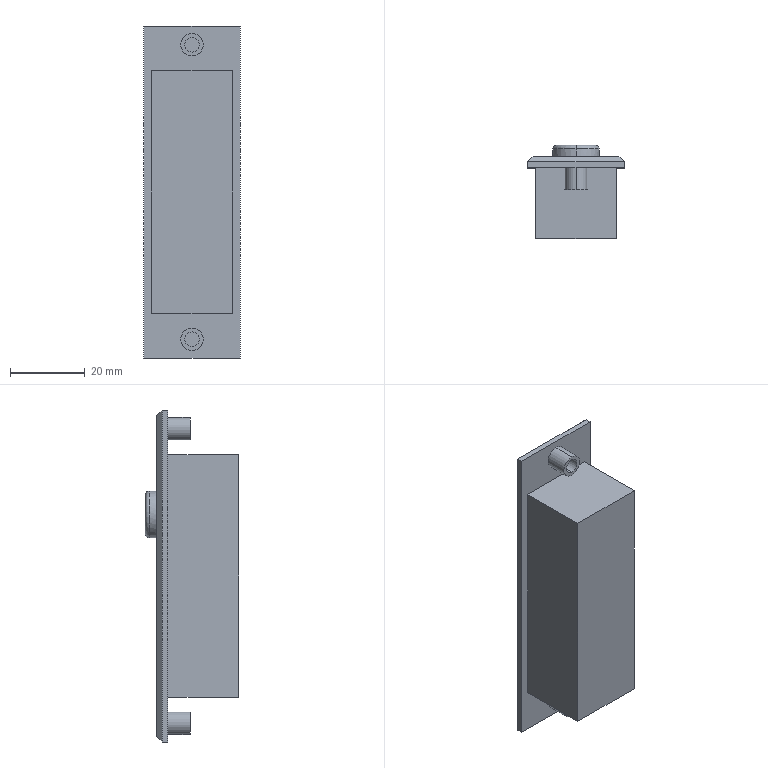Part | SolidWorks | features ICE 2, BossThin 1, Chamfer 1, CutThin 1, Extrusion 1, Fillet 1 | 1 solid | 45 faces | box 26 x 25 x 89 mm | volume 33780 mm3 | plane 29 | cylinder 10 | cone 4 | torus 2 | commonest cylinder face diameters 4 x4 6 x4 12.5 x2
STEP:
#1=CARTESIAN_POINT('',(0.,-6.,41.5));
#2=VERTEX_POINT('',#1);
#3=CARTESIAN_POINT('',(0.,-6.,37.5));
#4=VERTEX_POINT('',#3);
#5=CARTESIAN_POINT('',(0.,-6.,39.5));
#6=DIRECTION('',(0.,-1.,0.));
#7=DIRECTION('',(1.,0.,0.));
#8=AXIS2_PLACEMENT_3D('',#5,#6,#7);
#9=CIRCLE('',#8,2.);
#10=EDGE_CURVE('',#2,#4,#9,.T.);
#11=ORIENTED_EDGE('',*,*,#10,.T.);
#12=CARTESIAN_POINT('',(0.,0.,37.5));
#13=VERTEX_POINT('',#12);
#14=CARTESIAN_POINT('',(0.,-6.,37.5));
#15=DIRECTION('',(0.,1.,0.));
#16=VECTOR('',#15,1000.);
#17=LINE('',#14,#16);
#18=EDGE_CURVE('',#4,#13,#17,.T.);
#19=ORIENTED_EDGE('',*,*,#18,.T.);
#20=CARTESIAN_POINT('',(0.,0.,41.5));
#21=VERTEX_POINT('',#20);
#22=CARTESIAN_POINT('',(0.,0.,39.5));
#23=DIRECTION('',(0.,-1.,0.));
#24=DIRECTION('',(1.,0.,0.));
#25=AXIS2_PLACEMENT_3D('',#22,#23,#24);
#26=CIRCLE('',#25,2.);
#27=EDGE_CURVE('',#21,#13,#26,.T.);
#28=ORIENTED_EDGE('',*,*,#27,.F.);
#29=CARTESIAN_POINT('',(0.,-6.,41.5));
#30=DIRECTION('',(0.,1.,0.));
#31=VECTOR('',#30,1000.);
#32=LINE('',#29,#31);
#33=EDGE_CURVE('',#2,#21,#32,.T.);
#34=ORIENTED_EDGE('',*,*,#33,.F.);
#35=EDGE_LOOP('',(#11,#19,#28,#34));
#36=FACE_OUTER_BOUND('',#35,.T.);
#37=CARTESIAN_POINT('',(0.,-6.,39.5));
#38=DIRECTION('',(0.,1.,0.));
#39=DIRECTION('',(0.,0.,1.));
#40=AXIS2_PLACEMENT_3D('',#37,#38,#39);
#41=CYLINDRICAL_SURFACE('',#40,2.);
#42=ADVANCED_FACE('',(#36),#41,.F.);
#43=CARTESIAN_POINT('',(0.,-6.,36.5));
#44=VERTEX_POINT('',#43);
#45=CARTESIAN_POINT('',(0.,-6.,42.5));
#46=VERTEX_POINT('',#45);
#47=CARTESIAN_POINT('',(0.,-6.,39.5));
#48=DIRECTION('',(0.,-1.,0.));
#49=DIRECTION('',(0.,0.,-1.));
#50=AXIS2_PLACEMENT_3D('',#47,#48,#49);
#51=CIRCLE('',#50,3.);
#52=EDGE_CURVE('',#44,#46,#51,.T.);
#53=ORIENTED_EDGE('',*,*,#52,.F.);
#54=CARTESIAN_POINT('',(0.,0.,36.5));
#55=VERTEX_POINT('',#54);
#56=CARTESIAN_POINT('',(0.,-6.,36.5));
#57=DIRECTION('',(0.,1.,0.));
#58=VECTOR('',#57,1000.);
#59=LINE('',#56,#58);
#60=EDGE_CURVE('',#44,#55,#59,.T.);
#61=ORIENTED_EDGE('',*,*,#60,.T.);
#62=CARTESIAN_POINT('',(0.,0.,42.5));
#63=VERTEX_POINT('',#62);
#64=CARTESIAN_POINT('',(0.,0.,39.5));
#65=DIRECTION('',(0.,-1.,0.));
#66=DIRECTION('',(0.,0.,1.));
#67=AXIS2_PLACEMENT_3D('',#64,#65,#66);
#68=CIRCLE('',#67,3.);
#69=EDGE_CURVE('',#55,#63,#68,.T.);
#70=ORIENTED_EDGE('',*,*,#69,.T.);
#71=CARTESIAN_POINT('',(0.,-6.,42.5));
#72=DIRECTION('',(0.,1.,0.));
#73=VECTOR('',#72,1000.);
#74=LINE('',#71,#73);
#75=EDGE_CURVE('',#46,#63,#74,.T.);
#76=ORIENTED_EDGE('',*,*,#75,.F.);
#77=EDGE_LOOP('',(#53,#61,#70,#76));
#78=FACE_OUTER_BOUND('',#77,.T.);
#79=CARTESIAN_POINT('',(0.,-6.,39.5));
#80=DIRECTION('',(0.,1.,0.));
#81=DIRECTION('',(0.,0.,1.));
#82=AXIS2_PLACEMENT_3D('',#79,#80,#81);
#83=CYLINDRICAL_SURFACE('',#82,3.);
#84=ADVANCED_FACE('',(#78),#83,.T.);
#85=CARTESIAN_POINT('',(0.,-6.,-37.5));
#86=VERTEX_POINT('',#85);
#87=CARTESIAN_POINT('',(0.,-6.,-41.5));
#88=VERTEX_POINT('',#87);
#89=CARTESIAN_POINT('',(0.,-6.,-39.5));
#90=DIRECTION('',(0.,-1.,0.));
#91=DIRECTION('',(1.,0.,0.));
#92=AXIS2_PLACEMENT_3D('',#89,#90,#91);
#93=CIRCLE('',#92,2.);
#94=EDGE_CURVE('',#86,#88,#93,.T.);
#95=ORIENTED_EDGE('',*,*,#94,.T.);
#96=CARTESIAN_POINT('',(0.,0.,-41.5));
#97=VERTEX_POINT('',#96);
#98=CARTESIAN_POINT('',(0.,-6.,-41.5));
#99=DIRECTION('',(0.,1.,0.));
#100=VECTOR('',#99,1000.);
#101=LINE('',#98,#100);
#102=EDGE_CURVE('',#88,#97,#101,.T.);
#103=ORIENTED_EDGE('',*,*,#102,.T.);
#104=CARTESIAN_POINT('',(0.,0.,-37.5));
#105=VERTEX_POINT('',#104);
#106=CARTESIAN_POINT('',(0.,0.,-39.5));
#107=DIRECTION('',(0.,-1.,0.));
#108=DIRECTION('',(1.,0.,0.));
#109=AXIS2_PLACEMENT_3D('',#106,#107,#108);
#110=CIRCLE('',#109,2.);
#111=EDGE_CURVE('',#105,#97,#110,.T.);
#112=ORIENTED_EDGE('',*,*,#111,.F.);
#113=CARTESIAN_POINT('',(0.,-6.,-37.5));
#114=DIRECTION('',(0.,1.,0.));
#115=VECTOR('',#114,1000.);
#116=LINE('',#113,#115);
#117=EDGE_CURVE('',#86,#105,#116,.T.);
#118=ORIENTED_EDGE('',*,*,#117,.F.);
#119=EDGE_LOOP('',(#95,#103,#112,#118));
#120=FACE_OUTER_BOUND('',#119,.T.);
#121=CARTESIAN_POINT('',(0.,-6.,-39.5));
#122=DIRECTION('',(0.,1.,0.));
#123=DIRECTION('',(0.,0.,1.));
#124=AXIS2_PLACEMENT_3D('',#121,#122,#123);
#125=CYLINDRICAL_SURFACE('',#124,2.);
#126=ADVANCED_FACE('',(#120),#125,.F.);
#127=CARTESIAN_POINT('',(0.,-6.,-42.5));
#128=VERTEX_POINT('',#127);
#129=CARTESIAN_POINT('',(0.,-6.,-36.5));
#130=VERTEX_POINT('',#129);
#131=CARTESIAN_POINT('',(0.,-6.,-39.5));
#132=DIRECTION('',(0.,-1.,0.));
#133=DIRECTION('',(0.,0.,-1.));
#134=AXIS2_PLACEMENT_3D('',#131,#132,#133);
#135=CIRCLE('',#134,3.);
#136=EDGE_CURVE('',#128,#130,#135,.T.);
#137=ORIENTED_EDGE('',*,*,#136,.F.);
#138=CARTESIAN_POINT('',(0.,0.,-42.5));
#139=VERTEX_POINT('',#138);
#140=CARTESIAN_POINT('',(0.,-6.,-42.5));
#141=DIRECTION('',(0.,1.,0.));
#142=VECTOR('',#141,1000.);
#143=LINE('',#140,#142);
#144=EDGE_CURVE('',#128,#139,#143,.T.);
#145=ORIENTED_EDGE('',*,*,#144,.T.);
#146=CARTESIAN_POINT('',(0.,0.,-36.5));
#147=VERTEX_POINT('',#146);
#148=CARTESIAN_POINT('',(0.,0.,-39.5));
#149=DIRECTION('',(0.,-1.,0.));
#150=DIRECTION('',(0.,0.,1.));
#151=AXIS2_PLACEMENT_3D('',#148,#149,#150);
#152=CIRCLE('',#151,3.);
#153=EDGE_CURVE('',#139,#147,#152,.T.);
#154=ORIENTED_EDGE('',*,*,#153,.T.);
#155=CARTESIAN_POINT('',(0.,-6.,-36.5));
#156=DIRECTION('',(0.,1.,0.));
#157=VECTOR('',#156,1000.);
#158=LINE('',#155,#157);
#159=EDGE_CURVE('',#130,#147,#158,.T.);
#160=ORIENTED_EDGE('',*,*,#159,.F.);
#161=EDGE_LOOP('',(#137,#145,#154,#160));
#162=FACE_OUTER_BOUND('',#161,.T.);
#163=CARTESIAN_POINT('',(0.,-6.,-39.5));
#164=DIRECTION('',(0.,1.,0.));
#165=DIRECTION('',(0.,0.,1.));
#166=AXIS2_PLACEMENT_3D('',#163,#164,#165);
#167=CYLINDRICAL_SURFACE('',#166,3.);
#168=ADVANCED_FACE('',(#162),#167,.T.);
#169=CARTESIAN_POINT('',(0.,5.,10.25));
#170=VERTEX_POINT('',#169);
#171=CARTESIAN_POINT('',(0.,5.,22.75));
#172=VERTEX_POINT('',#171);
#173=CARTESIAN_POINT('',(0.,5.,16.5));
#174=DIRECTION('',(0.,-1.,0.));
#175=DIRECTION('',(0.,0.,1.));
#176=AXIS2_PLACEMENT_3D('',#173,#174,#175);
#177=CIRCLE('',#176,6.25);
#178=EDGE_CURVE('',#170,#172,#177,.T.);
#179=ORIENTED_EDGE('',*,*,#178,.F.);
#180=CARTESIAN_POINT('',(0.,6.,11.25));
#181=VERTEX_POINT('',#180);
#182=CARTESIAN_POINT('',(0.,5.,11.25));
#183=DIRECTION('',(1.,0.,0.));
#184=DIRECTION('',(0.,0.,-1.));
#185=AXIS2_PLACEMENT_3D('',#182,#183,#184);
#186=CIRCLE('',#185,1.);
#187=EDGE_CURVE('',#170,#181,#186,.T.);
#188=ORIENTED_EDGE('',*,*,#187,.T.);
#189=CARTESIAN_POINT('',(0.,6.,21.75));
#190=VERTEX_POINT('',#189);
#191=CARTESIAN_POINT('',(0.,6.,16.5));
#192=DIRECTION('',(0.,1.,0.));
#193=DIRECTION('',(0.,0.,1.));
#194=AXIS2_PLACEMENT_3D('',#191,#192,#193);
#195=CIRCLE('',#194,5.25);
#196=EDGE_CURVE('',#190,#181,#195,.T.);
#197=ORIENTED_EDGE('',*,*,#196,.F.);
#198=CARTESIAN_POINT('',(0.,5.,21.75));
#199=DIRECTION('',(-1.,0.,0.));
#200=DIRECTION('',(0.,0.,1.));
#201=AXIS2_PLACEMENT_3D('',#198,#199,#200);
#202=CIRCLE('',#201,1.);
#203=EDGE_CURVE('',#172,#190,#202,.T.);
#204=ORIENTED_EDGE('',*,*,#203,.F.);
#205=EDGE_LOOP('',(#179,#188,#197,#204));
#206=FACE_OUTER_BOUND('',#205,.T.);
#207=CARTESIAN_POINT('',(0.,5.,16.5));
#208=DIRECTION('',(0.,1.,0.));
#209=DIRECTION('',(0.,0.,1.));
#210=AXIS2_PLACEMENT_3D('',#207,#208,#209);
#211=TOROIDAL_SURFACE('',#210,5.25,1.);
#212=ADVANCED_FACE('',(#206),#211,.T.);
#213=ORIENTED_EDGE('',*,*,#178,.T.);
#214=CARTESIAN_POINT('',(0.,3.,22.75));
#215=VERTEX_POINT('',#214);
#216=CARTESIAN_POINT('',(0.,6.,22.75));
#217=DIRECTION('',(0.,-1.,0.));
#218=VECTOR('',#217,1000.);
#219=LINE('',#216,#218);
#220=EDGE_CURVE('',#172,#215,#219,.T.);
#221=ORIENTED_EDGE('',*,*,#220,.T.);
#222=CARTESIAN_POINT('',(6.25,3.,16.5));
#223=VERTEX_POINT('',#222);
#224=CARTESIAN_POINT('',(0.,3.,16.5));
#225=DIRECTION('',(0.,1.,0.));
#226=DIRECTION('',(1.,0.,0.));
#227=AXIS2_PLACEMENT_3D('',#224,#225,#226);
#228=CIRCLE('',#227,6.25);
#229=EDGE_CURVE('',#215,#223,#228,.T.);
#230=ORIENTED_EDGE('',*,*,#229,.T.);
#231=CARTESIAN_POINT('',(0.,3.,10.25));
#232=VERTEX_POINT('',#231);
#233=CARTESIAN_POINT('',(0.,3.,16.5));
#234=DIRECTION('',(0.,1.,0.));
#235=DIRECTION('',(1.,0.,0.));
#236=AXIS2_PLACEMENT_3D('',#233,#234,#235);
#237=CIRCLE('',#236,6.25);
#238=EDGE_CURVE('',#223,#232,#237,.T.);
#239=ORIENTED_EDGE('',*,*,#238,.T.);
#240=CARTESIAN_POINT('',(0.,6.,10.25));
#241=DIRECTION('',(0.,-1.,0.));
#242=VECTOR('',#241,1000.);
#243=LINE('',#240,#242);
#244=EDGE_CURVE('',#170,#232,#243,.T.);
#245=ORIENTED_EDGE('',*,*,#244,.F.);
#246=EDGE_LOOP('',(#213,#221,#230,#239,#245));
#247=FACE_OUTER_BOUND('',#246,.T.);
#248=CARTESIAN_POINT('',(0.,6.,16.5));
#249=DIRECTION('',(0.,-1.,0.));
#250=DIRECTION('',(0.,0.,-1.));
#251=AXIS2_PLACEMENT_3D('',#248,#249,#250);
#252=CYLINDRICAL_SURFACE('',#251,6.25);
#253=ADVANCED_FACE('',(#247),#252,.T.);
#254=CARTESIAN_POINT('',(-6.25,3.,16.5));
#255=VERTEX_POINT('',#254);
#256=CARTESIAN_POINT('',(0.,3.,16.5));
#257=DIRECTION('',(0.,1.,0.));
#258=DIRECTION('',(1.,0.,0.));
#259=AXIS2_PLACEMENT_3D('',#256,#257,#258);
#260=CIRCLE('',#259,6.25);
#261=EDGE_CURVE('',#255,#215,#260,.T.);
#262=ORIENTED_EDGE('',*,*,#261,.F.);
#263=CARTESIAN_POINT('',(-6.5,2.741,16.5));
#264=VERTEX_POINT('',#263);
#265=CARTESIAN_POINT('',(-6.25,3.,16.5));
#266=DIRECTION('',(-0.6947,-0.7193,0.));
#267=VECTOR('',#266,1000.);
#268=LINE('',#265,#267);
#269=EDGE_CURVE('',#255,#264,#268,.T.);
#270=ORIENTED_EDGE('',*,*,#269,.T.);
#271=CARTESIAN_POINT('',(6.5,2.741,16.5));
#272=VERTEX_POINT('',#271);
#273=CARTESIAN_POINT('',(0.,2.741,16.5));
#274=DIRECTION('',(0.,1.,0.));
#275=DIRECTION('',(0.,0.,1.));
#276=AXIS2_PLACEMENT_3D('',#273,#274,#275);
#277=CIRCLE('',#276,6.5);
#278=EDGE_CURVE('',#264,#272,#277,.T.);
#279=ORIENTED_EDGE('',*,*,#278,.T.);
#280=CARTESIAN_POINT('',(6.25,3.,16.5));
#281=DIRECTION('',(0.6947,-0.7193,0.));
#282=VECTOR('',#281,1000.);
#283=LINE('',#280,#282);
#284=EDGE_CURVE('',#223,#272,#283,.T.);
#285=ORIENTED_EDGE('',*,*,#284,.F.);
#286=ORIENTED_EDGE('',*,*,#229,.F.);
#287=EDGE_LOOP('',(#262,#270,#279,#285,#286));
#288=FACE_OUTER_BOUND('',#287,.T.);
#289=CARTESIAN_POINT('',(0.,3.,16.5));
#290=DIRECTION('',(0.,-1.,0.));
#291=DIRECTION('',(1.,0.,0.));
#292=AXIS2_PLACEMENT_3D('',#289,#290,#291);
#293=CONICAL_SURFACE('',#292,6.25,0.7679);
#294=ADVANCED_FACE('',(#288),#293,.T.);
#295=ORIENTED_EDGE('',*,*,#278,.F.);
#296=CARTESIAN_POINT('',(-6.75,3.,16.5));
#297=VERTEX_POINT('',#296);
#298=CARTESIAN_POINT('',(-6.75,3.,16.5));
#299=DIRECTION('',(-0.6947,0.7193,0.));
#300=VECTOR('',#299,1000.);
#301=LINE('',#298,#300);
#302=EDGE_CURVE('',#264,#297,#301,.T.);
#303=ORIENTED_EDGE('',*,*,#302,.T.);
#304=CARTESIAN_POINT('',(6.75,3.,16.5));
#305=VERTEX_POINT('',#304);
#306=CARTESIAN_POINT('',(0.,3.,16.5));
#307=DIRECTION('',(0.,1.,0.));
#308=DIRECTION('',(1.,0.,0.));
#309=AXIS2_PLACEMENT_3D('',#306,#307,#308);
#310=CIRCLE('',#309,6.75);
#311=EDGE_CURVE('',#297,#305,#310,.T.);
#312=ORIENTED_EDGE('',*,*,#311,.T.);
#313=CARTESIAN_POINT('',(6.75,3.,16.5));
#314=DIRECTION('',(0.6947,0.7193,0.));
#315=VECTOR('',#314,1000.);
#316=LINE('',#313,#315);
#317=EDGE_CURVE('',#272,#305,#316,.T.);
#318=ORIENTED_EDGE('',*,*,#317,.F.);
#319=EDGE_LOOP('',(#295,#303,#312,#318));
#320=FACE_OUTER_BOUND('',#319,.T.);
#321=CARTESIAN_POINT('',(0.,3.,16.5));
#322=DIRECTION('',(0.,1.,0.));
#323=DIRECTION('',(1.,0.,0.));
#324=AXIS2_PLACEMENT_3D('',#321,#322,#323);
#325=CONICAL_SURFACE('',#324,6.75,0.7679);
#326=ADVANCED_FACE('',(#320),#325,.F.);
#327=CARTESIAN_POINT('',(0.,0.,39.5));
#328=DIRECTION('',(0.,-1.,0.));
#329=DIRECTION('',(0.,0.,1.));
#330=AXIS2_PLACEMENT_3D('',#327,#328,#329);
#331=CIRCLE('',#330,3.);
#332=EDGE_CURVE('',#63,#55,#331,.T.);
#333=ORIENTED_EDGE('',*,*,#332,.F.);
#334=ORIENTED_EDGE('',*,*,#69,.F.);
#335=EDGE_LOOP('',(#333,#334));
#336=FACE_BOUND('',#335,.T.);
#337=CARTESIAN_POINT('',(0.,0.,-39.5));
#338=DIRECTION('',(0.,-1.,0.));
#339=DIRECTION('',(0.,0.,1.));
#340=AXIS2_PLACEMENT_3D('',#337,#338,#339);
#341=CIRCLE('',#340,3.);
#342=EDGE_CURVE('',#147,#139,#341,.T.);
#343=ORIENTED_EDGE('',*,*,#342,.F.);
#344=ORIENTED_EDGE('',*,*,#153,.F.);
#345=EDGE_LOOP('',(#343,#344));
#346=FACE_BOUND('',#345,.T.);
#347=CARTESIAN_POINT('',(13.,0.,44.5));
#348=VERTEX_POINT('',#347);
#349=CARTESIAN_POINT('',(13.,0.,-44.5));
#350=VERTEX_POINT('',#349);
#351=CARTESIAN_POINT('',(13.,0.,-44.5));
#352=DIRECTION('',(0.,0.,-1.));
#353=VECTOR('',#352,1000.);
#354=LINE('',#351,#353);
#355=EDGE_CURVE('',#348,#350,#354,.T.);
#356=ORIENTED_EDGE('',*,*,#355,.F.);
#357=CARTESIAN_POINT('',(-13.,0.,44.5));
#358=VERTEX_POINT('',#357);
#359=CARTESIAN_POINT('',(-13.,0.,44.5));
#360=DIRECTION('',(1.,0.,0.));
#361=VECTOR('',#360,1000.);
#362=LINE('',#359,#361);
#363=EDGE_CURVE('',#358,#348,#362,.T.);
#364=ORIENTED_EDGE('',*,*,#363,.F.);
#365=CARTESIAN_POINT('',(-13.,0.,-44.5));
#366=VERTEX_POINT('',#365);
#367=CARTESIAN_POINT('',(-13.,0.,-44.5));
#368=DIRECTION('',(0.,0.,1.));
#369=VECTOR('',#368,1000.);
#370=LINE('',#367,#369);
#371=EDGE_CURVE('',#366,#358,#370,.T.);
#372=ORIENTED_EDGE('',*,*,#371,.F.);
#373=CARTESIAN_POINT('',(-13.,0.,-44.5));
#374=DIRECTION('',(-1.,0.,0.));
#375=VECTOR('',#374,1000.);
#376=LINE('',#373,#375);
#377=EDGE_CURVE('',#350,#366,#376,.T.);
#378=ORIENTED_EDGE('',*,*,#377,.F.);
#379=EDGE_LOOP('',(#356,#364,#372,#378));
#380=FACE_OUTER_BOUND('',#379,.T.);
#381=CARTESIAN_POINT('',(-10.75,0.,32.5));
#382=VERTEX_POINT('',#381);
#383=CARTESIAN_POINT('',(-10.75,0.,-32.5));
#384=VERTEX_POINT('',#383);
#385=CARTESIAN_POINT('',(-10.75,0.,-32.5));
#386=DIRECTION('',(0.,0.,-1.));
#387=VECTOR('',#386,1000.);
#388=LINE('',#385,#387);
#389=EDGE_CURVE('',#382,#384,#388,.T.);
#390=ORIENTED_EDGE('',*,*,#389,.F.);
#391=CARTESIAN_POINT('',(10.75,0.,32.5));
#392=VERTEX_POINT('',#391);
#393=CARTESIAN_POINT('',(10.75,0.,32.5));
#394=DIRECTION('',(-1.,0.,0.));
#395=VECTOR('',#394,1000.);
#396=LINE('',#393,#395);
#397=EDGE_CURVE('',#392,#382,#396,.T.);
#398=ORIENTED_EDGE('',*,*,#397,.F.);
#399=CARTESIAN_POINT('',(10.75,0.,-32.5));
#400=VERTEX_POINT('',#399);
#401=CARTESIAN_POINT('',(10.75,0.,-32.5));
#402=DIRECTION('',(0.,0.,1.));
#403=VECTOR('',#402,1000.);
#404=LINE('',#401,#403);
#405=EDGE_CURVE('',#400,#392,#404,.T.);
#406=ORIENTED_EDGE('',*,*,#405,.F.);
#407=CARTESIAN_POINT('',(10.75,0.,-32.5));
#408=DIRECTION('',(1.,0.,0.));
#409=VECTOR('',#408,1000.);
#410=LINE('',#407,#409);
#411=EDGE_CURVE('',#384,#400,#410,.T.);
#412=ORIENTED_EDGE('',*,*,#411,.F.);
#413=EDGE_LOOP('',(#390,#398,#406,#412));
#414=FACE_BOUND('',#413,.T.);
#415=CARTESIAN_POINT('',(0.,0.,0.));
#416=DIRECTION('',(0.,1.,0.));
#417=DIRECTION('',(0.,0.,1.));
#418=AXIS2_PLACEMENT_3D('',#415,#416,#417);
#419=PLANE('',#418);
#420=ADVANCED_FACE('',(#336,#346,#380,#414),#419,.F.);
#421=CARTESIAN_POINT('',(13.,1.5,-44.5));
#422=VERTEX_POINT('',#421);
#423=CARTESIAN_POINT('',(13.,3.,-44.5));
#424=DIRECTION('',(0.,-1.,0.));
#425=VECTOR('',#424,1000.);
#426=LINE('',#423,#425);
#427=EDGE_CURVE('',#422,#350,#426,.T.);
#428=ORIENTED_EDGE('',*,*,#427,.F.);
#429=CARTESIAN_POINT('',(13.,1.5,44.5));
#430=VERTEX_POINT('',#429);
#431=CARTESIAN_POINT('',(13.,1.5,44.5));
#432=DIRECTION('',(0.,0.,1.));
#433=VECTOR('',#432,1000.);
#434=LINE('',#431,#433);
#435=EDGE_CURVE('',#422,#430,#434,.T.);
#436=ORIENTED_EDGE('',*,*,#435,.T.);
#437=CARTESIAN_POINT('',(13.,3.,44.5));
#438=DIRECTION('',(0.,-1.,0.));
#439=VECTOR('',#438,1000.);
#440=LINE('',#437,#439);
#441=EDGE_CURVE('',#430,#348,#440,.T.);
#442=ORIENTED_EDGE('',*,*,#441,.T.);
#443=ORIENTED_EDGE('',*,*,#355,.T.);
#444=EDGE_LOOP('',(#428,#436,#442,#443));
#445=FACE_OUTER_BOUND('',#444,.T.);
#446=CARTESIAN_POINT('',(13.,3.,-44.5));
#447=DIRECTION('',(-1.,0.,0.));
#448=DIRECTION('',(0.,0.,1.));
#449=AXIS2_PLACEMENT_3D('',#446,#447,#448);
#450=PLANE('',#449);
#451=ADVANCED_FACE('',(#445),#450,.F.);
#452=CARTESIAN_POINT('',(-13.,1.5,-44.5));
#453=VERTEX_POINT('',#452);
#454=CARTESIAN_POINT('',(-13.,3.,-44.5));
#455=DIRECTION('',(0.,-1.,0.));
#456=VECTOR('',#455,1000.);
#457=LINE('',#454,#456);
#458=EDGE_CURVE('',#453,#366,#457,.T.);
#459=ORIENTED_EDGE('',*,*,#458,.F.);
#460=CARTESIAN_POINT('',(13.,1.5,-44.5));
#461=DIRECTION('',(1.,0.,0.));
#462=VECTOR('',#461,1000.);
#463=LINE('',#460,#462);
#464=EDGE_CURVE('',#453,#422,#463,.T.);
#465=ORIENTED_EDGE('',*,*,#464,.T.);
#466=ORIENTED_EDGE('',*,*,#427,.T.);
#467=ORIENTED_EDGE('',*,*,#377,.T.);
#468=EDGE_LOOP('',(#459,#465,#466,#467));
#469=FACE_OUTER_BOUND('',#468,.T.);
#470=CARTESIAN_POINT('',(-13.,3.,-44.5));
#471=DIRECTION('',(0.,0.,1.));
#472=DIRECTION('',(1.,0.,0.));
#473=AXIS2_PLACEMENT_3D('',#470,#471,#472);
#474=PLANE('',#473);
#475=ADVANCED_FACE('',(#469),#474,.F.);
#476=CARTESIAN_POINT('',(-13.,1.5,44.5));
#477=VERTEX_POINT('',#476);
#478=CARTESIAN_POINT('',(-13.,3.,44.5));
#479=DIRECTION('',(0.,-1.,0.));
#480=VECTOR('',#479,1000.);
#481=LINE('',#478,#480);
#482=EDGE_CURVE('',#477,#358,#481,.T.);
#483=ORIENTED_EDGE('',*,*,#482,.F.);
#484=CARTESIAN_POINT('',(-13.,1.5,-44.5));
#485=DIRECTION('',(0.,0.,-1.));
#486=VECTOR('',#485,1000.);
#487=LINE('',#484,#486);
#488=EDGE_CURVE('',#477,#453,#487,.T.);
#489=ORIENTED_EDGE('',*,*,#488,.T.);
#490=ORIENTED_EDGE('',*,*,#458,.T.);
#491=ORIENTED_EDGE('',*,*,#371,.T.);
#492=EDGE_LOOP('',(#483,#489,#490,#491));
#493=FACE_OUTER_BOUND('',#492,.T.);
#494=CARTESIAN_POINT('',(-13.,3.,-44.5));
#495=DIRECTION('',(1.,0.,0.));
#496=DIRECTION('',(0.,0.,-1.));
#497=AXIS2_PLACEMENT_3D('',#494,#495,#496);
#498=PLANE('',#497);
#499=ADVANCED_FACE('',(#493),#498,.F.);
#500=ORIENTED_EDGE('',*,*,#441,.F.);
#501=CARTESIAN_POINT('',(-13.,1.5,44.5));
#502=DIRECTION('',(-1.,0.,0.));
#503=VECTOR('',#502,1000.);
#504=LINE('',#501,#503);
#505=EDGE_CURVE('',#430,#477,#504,.T.);
#506=ORIENTED_EDGE('',*,*,#505,.T.);
#507=ORIENTED_EDGE('',*,*,#482,.T.);
#508=ORIENTED_EDGE('',*,*,#363,.T.);
#509=EDGE_LOOP('',(#500,#506,#507,#508));
#510=FACE_OUTER_BOUND('',#509,.T.);
#511=CARTESIAN_POINT('',(-13.,3.,44.5));
#512=DIRECTION('',(0.,0.,-1.));
#513=DIRECTION('',(-1.,0.,0.));
#514=AXIS2_PLACEMENT_3D('',#511,#512,#513);
#515=PLANE('',#514);
#516=ADVANCED_FACE('',(#510),#515,.F.);
#517=CARTESIAN_POINT('',(11.5,3.,43.));
#518=VERTEX_POINT('',#517);
#519=CARTESIAN_POINT('',(11.5,3.,-43.));
#520=VERTEX_POINT('',#519);
#521=CARTESIAN_POINT('',(11.5,3.,-44.5));
#522=DIRECTION('',(0.,0.,-1.));
#523=VECTOR('',#522,1000.);
#524=LINE('',#521,#523);
#525=EDGE_CURVE('',#518,#520,#524,.T.);
#526=ORIENTED_EDGE('',*,*,#525,.T.);
#527=CARTESIAN_POINT('',(-11.5,3.,-43.));
#528=VERTEX_POINT('',#527);
#529=CARTESIAN_POINT('',(-13.,3.,-43.));
#530=DIRECTION('',(-1.,0.,0.));
#531=VECTOR('',#530,1000.);
#532=LINE('',#529,#531);
#533=EDGE_CURVE('',#520,#528,#532,.T.);
#534=ORIENTED_EDGE('',*,*,#533,.T.);
#535=CARTESIAN_POINT('',(-11.5,3.,43.));
#536=VERTEX_POINT('',#535);
#537=CARTESIAN_POINT('',(-11.5,3.,44.5));
#538=DIRECTION('',(0.,0.,1.));
#539=VECTOR('',#538,1000.);
#540=LINE('',#537,#539);
#541=EDGE_CURVE('',#528,#536,#540,.T.);
#542=ORIENTED_EDGE('',*,*,#541,.T.);
#543=CARTESIAN_POINT('',(13.,3.,43.));
#544=DIRECTION('',(1.,0.,0.));
#545=VECTOR('',#544,1000.);
#546=LINE('',#543,#545);
#547=EDGE_CURVE('',#536,#518,#546,.T.);
#548=ORIENTED_EDGE('',*,*,#547,.T.);
#549=EDGE_LOOP('',(#526,#534,#542,#548));
#550=FACE_OUTER_BOUND('',#549,.T.);
#551=CARTESIAN_POINT('',(0.,3.,16.5));
#552=DIRECTION('',(0.,1.,0.));
#553=DIRECTION('',(1.,0.,0.));
#554=AXIS2_PLACEMENT_3D('',#551,#552,#553);
#555=CIRCLE('',#554,6.75);
#556=EDGE_CURVE('',#305,#297,#555,.T.);
#557=ORIENTED_EDGE('',*,*,#556,.F.);
#558=ORIENTED_EDGE('',*,*,#311,.F.);
#559=EDGE_LOOP('',(#557,#558));
#560=FACE_BOUND('',#559,.T.);
#561=CARTESIAN_POINT('',(9.25,3.,3.75));
#562=VERTEX_POINT('',#561);
#563=CARTESIAN_POINT('',(9.25,3.,-28.75));
#564=VERTEX_POINT('',#563);
#565=CARTESIAN_POINT('',(9.25,3.,-28.5));
#566=DIRECTION('',(0.,0.,-1.));
#567=VECTOR('',#566,1000.);
#568=LINE('',#565,#567);
#569=EDGE_CURVE('',#562,#564,#568,.T.);
#570=ORIENTED_EDGE('',*,*,#569,.F.);
#571=CARTESIAN_POINT('',(-9.25,3.,3.75));
#572=VERTEX_POINT('',#571);
#573=CARTESIAN_POINT('',(-9.,3.,3.75));
#574=DIRECTION('',(1.,0.,0.));
#575=VECTOR('',#574,1000.);
#576=LINE('',#573,#575);
#577=EDGE_CURVE('',#572,#562,#576,.T.);
#578=ORIENTED_EDGE('',*,*,#577,.F.);
#579=CARTESIAN_POINT('',(-9.25,3.,-28.75));
#580=VERTEX_POINT('',#579);
#581=CARTESIAN_POINT('',(-9.25,3.,-28.5));
#582=DIRECTION('',(0.,0.,1.));
#583=VECTOR('',#582,1000.);
#584=LINE('',#581,#583);
#585=EDGE_CURVE('',#580,#572,#584,.T.);
#586=ORIENTED_EDGE('',*,*,#585,.F.);
#587=CARTESIAN_POINT('',(-9.,3.,-28.75));
#588=DIRECTION('',(-1.,0.,0.));
#589=VECTOR('',#588,1000.);
#590=LINE('',#587,#589);
#591=EDGE_CURVE('',#564,#580,#590,.T.);
#592=ORIENTED_EDGE('',*,*,#591,.F.);
#593=EDGE_LOOP('',(#570,#578,#586,#592));
#594=FACE_BOUND('',#593,.T.);
#595=CARTESIAN_POINT('',(0.,3.,0.));
#596=DIRECTION('',(0.,1.,0.));
#597=DIRECTION('',(0.,0.,1.));
#598=AXIS2_PLACEMENT_3D('',#595,#596,#597);
#599=PLANE('',#598);
#600=ADVANCED_FACE('',(#550,#560,#594),#599,.T.);
#601=CARTESIAN_POINT('',(9.,2.741,3.5));
#602=VERTEX_POINT('',#601);
#603=CARTESIAN_POINT('',(3.31,-3.151,-2.19));
#604=DIRECTION('',(0.5705,0.5908,0.5705));
#605=VECTOR('',#604,1000.);
#606=LINE('',#603,#605);
#607=EDGE_CURVE('',#602,#562,#606,.T.);
#608=ORIENTED_EDGE('',*,*,#607,.T.);
#609=ORIENTED_EDGE('',*,*,#569,.T.);
#610=CARTESIAN_POINT('',(9.,2.741,-28.5));
#611=VERTEX_POINT('',#610);
#612=CARTESIAN_POINT('',(9.169,2.916,-28.669));
#613=DIRECTION('',(0.5705,0.5908,-0.5705));
#614=VECTOR('',#613,1000.);
#615=LINE('',#612,#614);
#616=EDGE_CURVE('',#611,#564,#615,.T.);
#617=ORIENTED_EDGE('',*,*,#616,.F.);
#618=CARTESIAN_POINT('',(9.,2.741,-28.5));
#619=DIRECTION('',(0.,0.,-1.));
#620=VECTOR('',#619,1000.);
#621=LINE('',#618,#620);
#622=EDGE_CURVE('',#602,#611,#621,.T.);
#623=ORIENTED_EDGE('',*,*,#622,.F.);
#624=EDGE_LOOP('',(#608,#609,#617,#623));
#625=FACE_OUTER_BOUND('',#624,.T.);
#626=CARTESIAN_POINT('',(9.25,3.,-28.5));
#627=DIRECTION('',(0.7193,-0.6947,0.));
#628=DIRECTION('',(0.6947,0.7193,0.));
#629=AXIS2_PLACEMENT_3D('',#626,#627,#628);
#630=PLANE('',#629);
#631=ADVANCED_FACE('',(#625),#630,.F.);
#632=CARTESIAN_POINT('',(-9.,2.741,3.5));
#633=VERTEX_POINT('',#632);
#634=CARTESIAN_POINT('',(1.247,-7.87,-6.747));
#635=DIRECTION('',(-0.5705,0.5908,0.5705));
#636=VECTOR('',#635,1000.);
#637=LINE('',#634,#636);
#638=EDGE_CURVE('',#633,#572,#637,.T.);
#639=ORIENTED_EDGE('',*,*,#638,.T.);
#640=ORIENTED_EDGE('',*,*,#577,.T.);
#641=ORIENTED_EDGE('',*,*,#607,.F.);
#642=CARTESIAN_POINT('',(-9.,2.741,3.5));
#643=DIRECTION('',(1.,0.,0.));
#644=VECTOR('',#643,1000.);
#645=LINE('',#642,#644);
#646=EDGE_CURVE('',#633,#602,#645,.T.);
#647=ORIENTED_EDGE('',*,*,#646,.F.);
#648=EDGE_LOOP('',(#639,#640,#641,#647));
#649=FACE_OUTER_BOUND('',#648,.T.);
#650=CARTESIAN_POINT('',(-9.,3.,3.75));
#651=DIRECTION('',(0.,-0.6947,0.7193));
#652=DIRECTION('',(0.,-0.7193,-0.6947));
#653=AXIS2_PLACEMENT_3D('',#650,#651,#652);
#654=PLANE('',#653);
#655=ADVANCED_FACE('',(#649),#654,.F.);
#656=CARTESIAN_POINT('',(-9.,2.741,-28.5));
#657=VERTEX_POINT('',#656);
#658=CARTESIAN_POINT('',(-9.169,2.916,-28.669));
#659=DIRECTION('',(-0.5705,0.5908,-0.5705));
#660=VECTOR('',#659,1000.);
#661=LINE('',#658,#660);
#662=EDGE_CURVE('',#657,#580,#661,.T.);
#663=ORIENTED_EDGE('',*,*,#662,.T.);
#664=ORIENTED_EDGE('',*,*,#585,.T.);
#665=ORIENTED_EDGE('',*,*,#638,.F.);
#666=CARTESIAN_POINT('',(-9.,2.741,-28.5));
#667=DIRECTION('',(0.,0.,1.));
#668=VECTOR('',#667,1000.);
#669=LINE('',#666,#668);
#670=EDGE_CURVE('',#657,#633,#669,.T.);
#671=ORIENTED_EDGE('',*,*,#670,.F.);
#672=EDGE_LOOP('',(#663,#664,#665,#671));
#673=FACE_OUTER_BOUND('',#672,.T.);
#674=CARTESIAN_POINT('',(-9.25,3.,-28.5));
#675=DIRECTION('',(-0.7193,-0.6947,0.));
#676=DIRECTION('',(0.6947,-0.7193,0.));
#677=AXIS2_PLACEMENT_3D('',#674,#675,#676);
#678=PLANE('',#677);
#679=ADVANCED_FACE('',(#673),#678,.F.);
#680=ORIENTED_EDGE('',*,*,#616,.T.);
#681=ORIENTED_EDGE('',*,*,#591,.T.);
#682=ORIENTED_EDGE('',*,*,#662,.F.);
#683=CARTESIAN_POINT('',(-9.,2.741,-28.5));
#684=DIRECTION('',(-1.,0.,0.));
#685=VECTOR('',#684,1000.);
#686=LINE('',#683,#685);
#687=EDGE_CURVE('',#611,#657,#686,.T.);
#688=ORIENTED_EDGE('',*,*,#687,.F.);
#689=EDGE_LOOP('',(#680,#681,#682,#688));
#690=FACE_OUTER_BOUND('',#689,.T.);
#691=CARTESIAN_POINT('',(-9.,3.,-28.75));
#692=DIRECTION('',(0.,-0.6947,-0.7193));
#693=DIRECTION('',(0.,0.7193,-0.6947));
#694=AXIS2_PLACEMENT_3D('',#691,#692,#693);
#695=PLANE('',#694);
#696=ADVANCED_FACE('',(#690),#695,.F.);
#697=ORIENTED_EDGE('',*,*,#622,.T.);
#698=CARTESIAN_POINT('',(8.75,3.,-28.25));
#699=VERTEX_POINT('',#698);
#700=CARTESIAN_POINT('',(8.831,2.916,-28.331));
#701=DIRECTION('',(-0.5705,0.5908,0.5705));
#702=VECTOR('',#701,1000.);
#703=LINE('',#700,#702);
#704=EDGE_CURVE('',#611,#699,#703,.T.);
#705=ORIENTED_EDGE('',*,*,#704,.T.);
#706=CARTESIAN_POINT('',(8.75,3.,3.25));
#707=VERTEX_POINT('',#706);
#708=CARTESIAN_POINT('',(8.75,3.,-28.5));
#709=DIRECTION('',(0.,0.,-1.));
#710=VECTOR('',#709,1000.);
#711=LINE('',#708,#710);
#712=EDGE_CURVE('',#707,#699,#711,.T.);
#713=ORIENTED_EDGE('',*,*,#712,.F.);
#714=CARTESIAN_POINT('',(2.973,8.983,-2.527));
#715=DIRECTION('',(-0.5705,0.5908,-0.5705));
#716=VECTOR('',#715,1000.);
#717=LINE('',#714,#716);
#718=EDGE_CURVE('',#602,#707,#717,.T.);
#719=ORIENTED_EDGE('',*,*,#718,.F.);
#720=EDGE_LOOP('',(#697,#705,#713,#719));
#721=FACE_OUTER_BOUND('',#720,.T.);
#722=CARTESIAN_POINT('',(8.75,3.,-28.5));
#723=DIRECTION('',(-0.7193,-0.6947,0.));
#724=DIRECTION('',(0.6947,-0.7193,0.));
#725=AXIS2_PLACEMENT_3D('',#722,#723,#724);
#726=PLANE('',#725);
#727=ADVANCED_FACE('',(#721),#726,.F.);
#728=ORIENTED_EDGE('',*,*,#646,.T.);
#729=ORIENTED_EDGE('',*,*,#718,.T.);
#730=CARTESIAN_POINT('',(-8.75,3.,3.25));
#731=VERTEX_POINT('',#730);
#732=CARTESIAN_POINT('',(-9.,3.,3.25));
#733=DIRECTION('',(1.,0.,0.));
#734=VECTOR('',#733,1000.);
#735=LINE('',#732,#734);
#736=EDGE_CURVE('',#731,#707,#735,.T.);
#737=ORIENTED_EDGE('',*,*,#736,.F.);
#738=CARTESIAN_POINT('',(1.584,13.701,-7.084));
#739=DIRECTION('',(0.5705,0.5908,-0.5705));
#740=VECTOR('',#739,1000.);
#741=LINE('',#738,#740);
#742=EDGE_CURVE('',#633,#731,#741,.T.);
#743=ORIENTED_EDGE('',*,*,#742,.F.);
#744=EDGE_LOOP('',(#728,#729,#737,#743));
#745=FACE_OUTER_BOUND('',#744,.T.);
#746=CARTESIAN_POINT('',(-9.,3.,3.25));
#747=DIRECTION('',(0.,-0.6947,-0.7193));
#748=DIRECTION('',(0.,0.7193,-0.6947));
#749=AXIS2_PLACEMENT_3D('',#746,#747,#748);
#750=PLANE('',#749);
#751=ADVANCED_FACE('',(#745),#750,.F.);
#752=ORIENTED_EDGE('',*,*,#670,.T.);
#753=ORIENTED_EDGE('',*,*,#742,.T.);
#754=CARTESIAN_POINT('',(-8.75,3.,-28.25));
#755=VERTEX_POINT('',#754);
#756=CARTESIAN_POINT('',(-8.75,3.,-28.5));
#757=DIRECTION('',(0.,0.,1.));
#758=VECTOR('',#757,1000.);
#759=LINE('',#756,#758);
#760=EDGE_CURVE('',#755,#731,#759,.T.);
#761=ORIENTED_EDGE('',*,*,#760,.F.);
#762=CARTESIAN_POINT('',(-8.831,2.916,-28.331));
#763=DIRECTION('',(0.5705,0.5908,0.5705));
#764=VECTOR('',#763,1000.);
#765=LINE('',#762,#764);
#766=EDGE_CURVE('',#657,#755,#765,.T.);
#767=ORIENTED_EDGE('',*,*,#766,.F.);
#768=EDGE_LOOP('',(#752,#753,#761,#767));
#769=FACE_OUTER_BOUND('',#768,.T.);
#770=CARTESIAN_POINT('',(-8.75,3.,-28.5));
#771=DIRECTION('',(0.7193,-0.6947,0.));
#772=DIRECTION('',(0.6947,0.7193,0.));
#773=AXIS2_PLACEMENT_3D('',#770,#771,#772);
#774=PLANE('',#773);
#775=ADVANCED_FACE('',(#769),#774,.F.);
#776=ORIENTED_EDGE('',*,*,#687,.T.);
#777=ORIENTED_EDGE('',*,*,#766,.T.);
#778=CARTESIAN_POINT('',(-9.,3.,-28.25));
#779=DIRECTION('',(-1.,0.,0.));
#780=VECTOR('',#779,1000.);
#781=LINE('',#778,#780);
#782=EDGE_CURVE('',#699,#755,#781,.T.);
#783=ORIENTED_EDGE('',*,*,#782,.F.);
#784=ORIENTED_EDGE('',*,*,#704,.F.);
#785=EDGE_LOOP('',(#776,#777,#783,#784));
#786=FACE_OUTER_BOUND('',#785,.T.);
#787=CARTESIAN_POINT('',(-9.,3.,-28.25));
#788=DIRECTION('',(0.,-0.6947,0.7193));
#789=DIRECTION('',(0.,-0.7193,-0.6947));
#790=AXIS2_PLACEMENT_3D('',#787,#788,#789);
#791=PLANE('',#790);
#792=ADVANCED_FACE('',(#786),#791,.F.);
#793=ORIENTED_EDGE('',*,*,#736,.T.);
#794=ORIENTED_EDGE('',*,*,#712,.T.);
#795=ORIENTED_EDGE('',*,*,#782,.T.);
#796=ORIENTED_EDGE('',*,*,#760,.T.);
#797=EDGE_LOOP('',(#793,#794,#795,#796));
#798=FACE_OUTER_BOUND('',#797,.T.);
#799=CARTESIAN_POINT('',(0.,3.,0.));
#800=DIRECTION('',(0.,1.,0.));
#801=DIRECTION('',(0.,0.,1.));
#802=AXIS2_PLACEMENT_3D('',#799,#800,#801);
#803=PLANE('',#802);
#804=ADVANCED_FACE('',(#798),#803,.T.);
#805=ORIENTED_EDGE('',*,*,#302,.F.);
#806=CARTESIAN_POINT('',(0.,2.741,16.5));
#807=DIRECTION('',(0.,1.,0.));
#808=DIRECTION('',(0.,0.,1.));
#809=AXIS2_PLACEMENT_3D('',#806,#807,#808);
#810=CIRCLE('',#809,6.5);
#811=EDGE_CURVE('',#272,#264,#810,.T.);
#812=ORIENTED_EDGE('',*,*,#811,.F.);
#813=ORIENTED_EDGE('',*,*,#317,.T.);
#814=ORIENTED_EDGE('',*,*,#556,.T.);
#815=EDGE_LOOP('',(#805,#812,#813,#814));
#816=FACE_OUTER_BOUND('',#815,.T.);
#817=CARTESIAN_POINT('',(0.,3.,16.5));
#818=DIRECTION('',(0.,1.,0.));
#819=DIRECTION('',(1.,0.,0.));
#820=AXIS2_PLACEMENT_3D('',#817,#818,#819);
#821=CONICAL_SURFACE('',#820,6.75,0.7679);
#822=ADVANCED_FACE('',(#816),#821,.F.);
#823=ORIENTED_EDGE('',*,*,#269,.F.);
#824=CARTESIAN_POINT('',(0.,3.,16.5));
#825=DIRECTION('',(0.,1.,0.));
#826=DIRECTION('',(1.,0.,0.));
#827=AXIS2_PLACEMENT_3D('',#824,#825,#826);
#828=CIRCLE('',#827,6.25);
#829=EDGE_CURVE('',#232,#255,#828,.T.);
#830=ORIENTED_EDGE('',*,*,#829,.F.);
#831=ORIENTED_EDGE('',*,*,#238,.F.);
#832=ORIENTED_EDGE('',*,*,#284,.T.);
#833=ORIENTED_EDGE('',*,*,#811,.T.);
#834=EDGE_LOOP('',(#823,#830,#831,#832,#833));
#835=FACE_OUTER_BOUND('',#834,.T.);
#836=CARTESIAN_POINT('',(0.,3.,16.5));
#837=DIRECTION('',(0.,-1.,0.));
#838=DIRECTION('',(1.,0.,0.));
#839=AXIS2_PLACEMENT_3D('',#836,#837,#838);
#840=CONICAL_SURFACE('',#839,6.25,0.7679);
#841=ADVANCED_FACE('',(#835),#840,.T.);
#842=ORIENTED_EDGE('',*,*,#220,.F.);
#843=CARTESIAN_POINT('',(0.,5.,16.5));
#844=DIRECTION('',(0.,-1.,0.));
#845=DIRECTION('',(0.,0.,1.));
#846=AXIS2_PLACEMENT_3D('',#843,#844,#845);
#847=CIRCLE('',#846,6.25);
#848=EDGE_CURVE('',#172,#170,#847,.T.);
#849=ORIENTED_EDGE('',*,*,#848,.T.);
#850=ORIENTED_EDGE('',*,*,#244,.T.);
#851=ORIENTED_EDGE('',*,*,#829,.T.);
#852=ORIENTED_EDGE('',*,*,#261,.T.);
#853=EDGE_LOOP('',(#842,#849,#850,#851,#852));
#854=FACE_OUTER_BOUND('',#853,.T.);
#855=CARTESIAN_POINT('',(0.,6.,16.5));
#856=DIRECTION('',(0.,-1.,0.));
#857=DIRECTION('',(0.,0.,-1.));
#858=AXIS2_PLACEMENT_3D('',#855,#856,#857);
#859=CYLINDRICAL_SURFACE('',#858,6.25);
#860=ADVANCED_FACE('',(#854),#859,.T.);
#861=ORIENTED_EDGE('',*,*,#196,.T.);
#862=CARTESIAN_POINT('',(0.,6.,16.5));
#863=DIRECTION('',(0.,1.,0.));
#864=DIRECTION('',(0.,0.,1.));
#865=AXIS2_PLACEMENT_3D('',#862,#863,#864);
#866=CIRCLE('',#865,5.25);
#867=EDGE_CURVE('',#181,#190,#866,.T.);
#868=ORIENTED_EDGE('',*,*,#867,.T.);
#869=EDGE_LOOP('',(#861,#868));
#870=FACE_OUTER_BOUND('',#869,.T.);
#871=CARTESIAN_POINT('',(0.,6.,16.5));
#872=DIRECTION('',(0.,1.,0.));
#873=DIRECTION('',(0.,0.,1.));
#874=AXIS2_PLACEMENT_3D('',#871,#872,#873);
#875=PLANE('',#874);
#876=ADVANCED_FACE('',(#870),#875,.T.);
#877=ORIENTED_EDGE('',*,*,#187,.F.);
#878=ORIENTED_EDGE('',*,*,#848,.F.);
#879=ORIENTED_EDGE('',*,*,#203,.T.);
#880=ORIENTED_EDGE('',*,*,#867,.F.);
#881=EDGE_LOOP('',(#877,#878,#879,#880));
#882=FACE_OUTER_BOUND('',#881,.T.);
#883=CARTESIAN_POINT('',(0.,5.,16.5));
#884=DIRECTION('',(0.,1.,0.));
#885=DIRECTION('',(0.,0.,1.));
#886=AXIS2_PLACEMENT_3D('',#883,#884,#885);
#887=TOROIDAL_SURFACE('',#886,5.25,1.);
#888=ADVANCED_FACE('',(#882),#887,.T.);
#889=CARTESIAN_POINT('',(2.833,17.333,28.667));
#890=DIRECTION('',(0.5774,0.5774,-0.5774));
#891=VECTOR('',#890,1000.);
#892=LINE('',#889,#891);
#893=EDGE_CURVE('',#477,#536,#892,.T.);
#894=ORIENTED_EDGE('',*,*,#893,.F.);
#895=ORIENTED_EDGE('',*,*,#505,.F.);
#896=CARTESIAN_POINT('',(7.667,6.833,39.167));
#897=DIRECTION('',(0.5774,-0.5774,0.5774));
#898=VECTOR('',#897,1000.);
#899=LINE('',#896,#898);
#900=EDGE_CURVE('',#518,#430,#899,.T.);
#901=ORIENTED_EDGE('',*,*,#900,.F.);
#902=ORIENTED_EDGE('',*,*,#547,.F.);
#903=EDGE_LOOP('',(#894,#895,#901,#902));
#904=FACE_OUTER_BOUND('',#903,.T.);
#905=CARTESIAN_POINT('',(0.,3.,43.));
#906=DIRECTION('',(0.,0.7071,0.7071));
#907=DIRECTION('',(-1.,0.,0.));
#908=AXIS2_PLACEMENT_3D('',#905,#906,#907);
#909=PLANE('',#908);
#910=ADVANCED_FACE('',(#904),#909,.T.);
#911=ORIENTED_EDGE('',*,*,#900,.T.);
#912=ORIENTED_EDGE('',*,*,#435,.F.);
#913=CARTESIAN_POINT('',(-2.833,17.333,-28.667));
#914=DIRECTION('',(0.5774,-0.5774,-0.5774));
#915=VECTOR('',#914,1000.);
#916=LINE('',#913,#915);
#917=EDGE_CURVE('',#520,#422,#916,.T.);
#918=ORIENTED_EDGE('',*,*,#917,.F.);
#919=ORIENTED_EDGE('',*,*,#525,.F.);
#920=EDGE_LOOP('',(#911,#912,#918,#919));
#921=FACE_OUTER_BOUND('',#920,.T.);
#922=CARTESIAN_POINT('',(11.5,3.,0.));
#923=DIRECTION('',(0.7071,0.7071,0.));
#924=DIRECTION('',(0.,0.,1.));
#925=AXIS2_PLACEMENT_3D('',#922,#923,#924);
#926=PLANE('',#925);
#927=ADVANCED_FACE('',(#921),#926,.T.);
#928=ORIENTED_EDGE('',*,*,#893,.T.);
#929=ORIENTED_EDGE('',*,*,#541,.F.);
#930=CARTESIAN_POINT('',(2.833,17.333,-28.667));
#931=DIRECTION('',(0.5774,0.5774,0.5774));
#932=VECTOR('',#931,1000.);
#933=LINE('',#930,#932);
#934=EDGE_CURVE('',#453,#528,#933,.T.);
#935=ORIENTED_EDGE('',*,*,#934,.F.);
#936=ORIENTED_EDGE('',*,*,#488,.F.);
#937=EDGE_LOOP('',(#928,#929,#935,#936));
#938=FACE_OUTER_BOUND('',#937,.T.);
#939=CARTESIAN_POINT('',(-11.5,3.,0.));
#940=DIRECTION('',(-0.7071,0.7071,0.));
#941=DIRECTION('',(0.,0.,-1.));
#942=AXIS2_PLACEMENT_3D('',#939,#940,#941);
#943=PLANE('',#942);
#944=ADVANCED_FACE('',(#938),#943,.T.);
#945=ORIENTED_EDGE('',*,*,#917,.T.);
#946=ORIENTED_EDGE('',*,*,#464,.F.);
#947=ORIENTED_EDGE('',*,*,#934,.T.);
#948=ORIENTED_EDGE('',*,*,#533,.F.);
#949=EDGE_LOOP('',(#945,#946,#947,#948));
#950=FACE_OUTER_BOUND('',#949,.T.);
#951=CARTESIAN_POINT('',(0.,3.,-43.));
#952=DIRECTION('',(0.,0.7071,-0.7071));
#953=DIRECTION('',(1.,0.,0.));
#954=AXIS2_PLACEMENT_3D('',#951,#952,#953);
#955=PLANE('',#954);
#956=ADVANCED_FACE('',(#950),#955,.T.);
#957=CARTESIAN_POINT('',(0.,-6.,-39.5));
#958=DIRECTION('',(0.,-1.,0.));
#959=DIRECTION('',(0.,0.,-1.));
#960=AXIS2_PLACEMENT_3D('',#957,#958,#959);
#961=CIRCLE('',#960,3.);
#962=EDGE_CURVE('',#130,#128,#961,.T.);
#963=ORIENTED_EDGE('',*,*,#962,.T.);
#964=ORIENTED_EDGE('',*,*,#136,.T.);
#965=EDGE_LOOP('',(#963,#964));
#966=FACE_OUTER_BOUND('',#965,.T.);
#967=ORIENTED_EDGE('',*,*,#94,.F.);
#968=CARTESIAN_POINT('',(0.,-6.,-39.5));
#969=DIRECTION('',(0.,-1.,0.));
#970=DIRECTION('',(1.,0.,0.));
#971=AXIS2_PLACEMENT_3D('',#968,#969,#970);
#972=CIRCLE('',#971,2.);
#973=EDGE_CURVE('',#88,#86,#972,.T.);
#974=ORIENTED_EDGE('',*,*,#973,.F.);
#975=EDGE_LOOP('',(#967,#974));
#976=FACE_BOUND('',#975,.T.);
#977=CARTESIAN_POINT('',(0.,-6.,-39.5));
#978=DIRECTION('',(0.,-1.,0.));
#979=DIRECTION('',(0.,0.,-1.));
#980=AXIS2_PLACEMENT_3D('',#977,#978,#979);
#981=PLANE('',#980);
#982=ADVANCED_FACE('',(#966,#976),#981,.T.);
#983=ORIENTED_EDGE('',*,*,#144,.F.);
#984=ORIENTED_EDGE('',*,*,#962,.F.);
#985=ORIENTED_EDGE('',*,*,#159,.T.);
#986=ORIENTED_EDGE('',*,*,#342,.T.);
#987=EDGE_LOOP('',(#983,#984,#985,#986));
#988=FACE_OUTER_BOUND('',#987,.T.);
#989=CARTESIAN_POINT('',(0.,-6.,-39.5));
#990=DIRECTION('',(0.,1.,0.));
#991=DIRECTION('',(0.,0.,1.));
#992=AXIS2_PLACEMENT_3D('',#989,#990,#991);
#993=CYLINDRICAL_SURFACE('',#992,3.);
#994=ADVANCED_FACE('',(#988),#993,.T.);
#995=ORIENTED_EDGE('',*,*,#102,.F.);
#996=ORIENTED_EDGE('',*,*,#973,.T.);
#997=ORIENTED_EDGE('',*,*,#117,.T.);
#998=CARTESIAN_POINT('',(0.,0.,-39.5));
#999=DIRECTION('',(0.,-1.,0.));
#1000=DIRECTION('',(1.,0.,0.));
#1001=AXIS2_PLACEMENT_3D('',#998,#999,#1000);
#1002=CIRCLE('',#1001,2.);
#1003=EDGE_CURVE('',#97,#105,#1002,.T.);
#1004=ORIENTED_EDGE('',*,*,#1003,.F.);
#1005=EDGE_LOOP('',(#995,#996,#997,#1004));
#1006=FACE_OUTER_BOUND('',#1005,.T.);
#1007=CARTESIAN_POINT('',(0.,-6.,-39.5));
#1008=DIRECTION('',(0.,1.,0.));
#1009=DIRECTION('',(0.,0.,1.));
#1010=AXIS2_PLACEMENT_3D('',#1007,#1008,#1009);
#1011=CYLINDRICAL_SURFACE('',#1010,2.);
#1012=ADVANCED_FACE('',(#1006),#1011,.F.);
#1013=ORIENTED_EDGE('',*,*,#111,.T.);
#1014=ORIENTED_EDGE('',*,*,#1003,.T.);
#1015=EDGE_LOOP('',(#1013,#1014));
#1016=FACE_OUTER_BOUND('',#1015,.T.);
#1017=CARTESIAN_POINT('',(0.,0.,0.));
#1018=DIRECTION('',(0.,1.,0.));
#1019=DIRECTION('',(0.,0.,1.));
#1020=AXIS2_PLACEMENT_3D('',#1017,#1018,#1019);
#1021=PLANE('',#1020);
#1022=ADVANCED_FACE('',(#1016),#1021,.F.);
#1023=CARTESIAN_POINT('',(0.,-6.,39.5));
#1024=DIRECTION('',(0.,-1.,0.));
#1025=DIRECTION('',(0.,0.,-1.));
#1026=AXIS2_PLACEMENT_3D('',#1023,#1024,#1025);
#1027=CIRCLE('',#1026,3.);
#1028=EDGE_CURVE('',#46,#44,#1027,.T.);
#1029=ORIENTED_EDGE('',*,*,#1028,.T.);
#1030=ORIENTED_EDGE('',*,*,#52,.T.);
#1031=EDGE_LOOP('',(#1029,#1030));
#1032=FACE_OUTER_BOUND('',#1031,.T.);
#1033=ORIENTED_EDGE('',*,*,#10,.F.);
#1034=CARTESIAN_POINT('',(0.,-6.,39.5));
#1035=DIRECTION('',(0.,-1.,0.));
#1036=DIRECTION('',(1.,0.,0.));
#1037=AXIS2_PLACEMENT_3D('',#1034,#1035,#1036);
#1038=CIRCLE('',#1037,2.);
#1039=EDGE_CURVE('',#4,#2,#1038,.T.);
#1040=ORIENTED_EDGE('',*,*,#1039,.F.);
#1041=EDGE_LOOP('',(#1033,#1040));
#1042=FACE_BOUND('',#1041,.T.);
#1043=CARTESIAN_POINT('',(0.,-6.,39.5));
#1044=DIRECTION('',(0.,-1.,0.));
#1045=DIRECTION('',(0.,0.,-1.));
#1046=AXIS2_PLACEMENT_3D('',#1043,#1044,#1045);
#1047=PLANE('',#1046);
#1048=ADVANCED_FACE('',(#1032,#1042),#1047,.T.);
#1049=ORIENTED_EDGE('',*,*,#60,.F.);
#1050=ORIENTED_EDGE('',*,*,#1028,.F.);
#1051=ORIENTED_EDGE('',*,*,#75,.T.);
#1052=ORIENTED_EDGE('',*,*,#332,.T.);
#1053=EDGE_LOOP('',(#1049,#1050,#1051,#1052));
#1054=FACE_OUTER_BOUND('',#1053,.T.);
#1055=CARTESIAN_POINT('',(0.,-6.,39.5));
#1056=DIRECTION('',(0.,1.,0.));
#1057=DIRECTION('',(0.,0.,1.));
#1058=AXIS2_PLACEMENT_3D('',#1055,#1056,#1057);
#1059=CYLINDRICAL_SURFACE('',#1058,3.);
#1060=ADVANCED_FACE('',(#1054),#1059,.T.);
#1061=ORIENTED_EDGE('',*,*,#18,.F.);
#1062=ORIENTED_EDGE('',*,*,#1039,.T.);
#1063=ORIENTED_EDGE('',*,*,#33,.T.);
#1064=CARTESIAN_POINT('',(0.,0.,39.5));
#1065=DIRECTION('',(0.,-1.,0.));
#1066=DIRECTION('',(1.,0.,0.));
#1067=AXIS2_PLACEMENT_3D('',#1064,#1065,#1066);
#1068=CIRCLE('',#1067,2.);
#1069=EDGE_CURVE('',#13,#21,#1068,.T.);
#1070=ORIENTED_EDGE('',*,*,#1069,.F.);
#1071=EDGE_LOOP('',(#1061,#1062,#1063,#1070));
#1072=FACE_OUTER_BOUND('',#1071,.T.);
#1073=CARTESIAN_POINT('',(0.,-6.,39.5));
#1074=DIRECTION('',(0.,1.,0.));
#1075=DIRECTION('',(0.,0.,1.));
#1076=AXIS2_PLACEMENT_3D('',#1073,#1074,#1075);
#1077=CYLINDRICAL_SURFACE('',#1076,2.);
#1078=ADVANCED_FACE('',(#1072),#1077,.F.);
#1079=ORIENTED_EDGE('',*,*,#27,.T.);
#1080=ORIENTED_EDGE('',*,*,#1069,.T.);
#1081=EDGE_LOOP('',(#1079,#1080));
#1082=FACE_OUTER_BOUND('',#1081,.T.);
#1083=CARTESIAN_POINT('',(0.,0.,0.));
#1084=DIRECTION('',(0.,1.,0.));
#1085=DIRECTION('',(0.,0.,1.));
#1086=AXIS2_PLACEMENT_3D('',#1083,#1084,#1085);
#1087=PLANE('',#1086);
#1088=ADVANCED_FACE('',(#1082),#1087,.F.);
#1089=ORIENTED_EDGE('',*,*,#389,.T.);
#1090=CARTESIAN_POINT('',(-10.75,-19.,-32.5));
#1091=VERTEX_POINT('',#1090);
#1092=CARTESIAN_POINT('',(-10.75,-19.,-32.5));
#1093=DIRECTION('',(0.,1.,0.));
#1094=VECTOR('',#1093,1000.);
#1095=LINE('',#1092,#1094);
#1096=EDGE_CURVE('',#1091,#384,#1095,.T.);
#1097=ORIENTED_EDGE('',*,*,#1096,.F.);
#1098=CARTESIAN_POINT('',(-10.75,-19.,32.5));
#1099=VERTEX_POINT('',#1098);
#1100=CARTESIAN_POINT('',(-10.75,-19.,-32.5));
#1101=DIRECTION('',(0.,0.,-1.));
#1102=VECTOR('',#1101,1000.);
#1103=LINE('',#1100,#1102);
#1104=EDGE_CURVE('',#1099,#1091,#1103,.T.);
#1105=ORIENTED_EDGE('',*,*,#1104,.F.);
#1106=CARTESIAN_POINT('',(-10.75,-19.,32.5));
#1107=DIRECTION('',(0.,1.,0.));
#1108=VECTOR('',#1107,1000.);
#1109=LINE('',#1106,#1108);
#1110=EDGE_CURVE('',#1099,#382,#1109,.T.);
#1111=ORIENTED_EDGE('',*,*,#1110,.T.);
#1112=EDGE_LOOP('',(#1089,#1097,#1105,#1111));
#1113=FACE_OUTER_BOUND('',#1112,.T.);
#1114=CARTESIAN_POINT('',(-10.75,-19.,-32.5));
#1115=DIRECTION('',(1.,0.,0.));
#1116=DIRECTION('',(0.,0.,-1.));
#1117=AXIS2_PLACEMENT_3D('',#1114,#1115,#1116);
#1118=PLANE('',#1117);
#1119=ADVANCED_FACE('',(#1113),#1118,.F.);
#1120=ORIENTED_EDGE('',*,*,#411,.T.);
#1121=CARTESIAN_POINT('',(10.75,-19.,-32.5));
#1122=VERTEX_POINT('',#1121);
#1123=CARTESIAN_POINT('',(10.75,-19.,-32.5));
#1124=DIRECTION('',(0.,1.,0.));
#1125=VECTOR('',#1124,1000.);
#1126=LINE('',#1123,#1125);
#1127=EDGE_CURVE('',#1122,#400,#1126,.T.);
#1128=ORIENTED_EDGE('',*,*,#1127,.F.);
#1129=CARTESIAN_POINT('',(10.75,-19.,-32.5));
#1130=DIRECTION('',(1.,0.,0.));
#1131=VECTOR('',#1130,1000.);
#1132=LINE('',#1129,#1131);
#1133=EDGE_CURVE('',#1091,#1122,#1132,.T.);
#1134=ORIENTED_EDGE('',*,*,#1133,.F.);
#1135=ORIENTED_EDGE('',*,*,#1096,.T.);
#1136=EDGE_LOOP('',(#1120,#1128,#1134,#1135));
#1137=FACE_OUTER_BOUND('',#1136,.T.);
#1138=CARTESIAN_POINT('',(10.75,-19.,-32.5));
#1139=DIRECTION('',(0.,0.,1.));
#1140=DIRECTION('',(1.,0.,0.));
#1141=AXIS2_PLACEMENT_3D('',#1138,#1139,#1140);
#1142=PLANE('',#1141);
#1143=ADVANCED_FACE('',(#1137),#1142,.F.);
#1144=ORIENTED_EDGE('',*,*,#405,.T.);
#1145=CARTESIAN_POINT('',(10.75,-19.,32.5));
#1146=VERTEX_POINT('',#1145);
#1147=CARTESIAN_POINT('',(10.75,-19.,32.5));
#1148=DIRECTION('',(0.,1.,0.));
#1149=VECTOR('',#1148,1000.);
#1150=LINE('',#1147,#1149);
#1151=EDGE_CURVE('',#1146,#392,#1150,.T.);
#1152=ORIENTED_EDGE('',*,*,#1151,.F.);
#1153=CARTESIAN_POINT('',(10.75,-19.,-32.5));
#1154=DIRECTION('',(0.,0.,1.));
#1155=VECTOR('',#1154,1000.);
#1156=LINE('',#1153,#1155);
#1157=EDGE_CURVE('',#1122,#1146,#1156,.T.);
#1158=ORIENTED_EDGE('',*,*,#1157,.F.);
#1159=ORIENTED_EDGE('',*,*,#1127,.T.);
#1160=EDGE_LOOP('',(#1144,#1152,#1158,#1159));
#1161=FACE_OUTER_BOUND('',#1160,.T.);
#1162=CARTESIAN_POINT('',(10.75,-19.,-32.5));
#1163=DIRECTION('',(-1.,0.,0.));
#1164=DIRECTION('',(0.,0.,1.));
#1165=AXIS2_PLACEMENT_3D('',#1162,#1163,#1164);
#1166=PLANE('',#1165);
#1167=ADVANCED_FACE('',(#1161),#1166,.F.);
#1168=ORIENTED_EDGE('',*,*,#397,.T.);
#1169=ORIENTED_EDGE('',*,*,#1110,.F.);
#1170=CARTESIAN_POINT('',(10.75,-19.,32.5));
#1171=DIRECTION('',(-1.,0.,0.));
#1172=VECTOR('',#1171,1000.);
#1173=LINE('',#1170,#1172);
#1174=EDGE_CURVE('',#1146,#1099,#1173,.T.);
#1175=ORIENTED_EDGE('',*,*,#1174,.F.);
#1176=ORIENTED_EDGE('',*,*,#1151,.T.);
#1177=EDGE_LOOP('',(#1168,#1169,#1175,#1176));
#1178=FACE_OUTER_BOUND('',#1177,.T.);
#1179=CARTESIAN_POINT('',(10.75,-19.,32.5));
#1180=DIRECTION('',(0.,0.,-1.));
#1181=DIRECTION('',(-1.,0.,0.));
#1182=AXIS2_PLACEMENT_3D('',#1179,#1180,#1181);
#1183=PLANE('',#1182);
#1184=ADVANCED_FACE('',(#1178),#1183,.F.);
#1185=ORIENTED_EDGE('',*,*,#1104,.T.);
#1186=ORIENTED_EDGE('',*,*,#1133,.T.);
#1187=ORIENTED_EDGE('',*,*,#1157,.T.);
#1188=ORIENTED_EDGE('',*,*,#1174,.T.);
#1189=EDGE_LOOP('',(#1185,#1186,#1187,#1188));
#1190=FACE_OUTER_BOUND('',#1189,.T.);
#1191=CARTESIAN_POINT('',(0.,-19.,0.));
#1192=DIRECTION('',(0.,-1.,0.));
#1193=DIRECTION('',(0.,0.,-1.));
#1194=AXIS2_PLACEMENT_3D('',#1191,#1192,#1193);
#1195=PLANE('',#1194);
#1196=ADVANCED_FACE('',(#1190),#1195,.T.);
#1197=CLOSED_SHELL('',(#42,#84,#126,#168,#212,#253,#294,#326,#420,#451,#475,#499,#516,#600,#631,#655,#679,#696,#727,#751,#775,#792,#804,#822,#841,#860,#876,#888,#910,#927,#944,#956,#982,#994,#1012,#1022,#1048,#1060,#1078,#1088,#1119,#1143,#1167,#1184,#1196));
#1198=MANIFOLD_SOLID_BREP('',#1197);
#1199=CARTESIAN_POINT('',(0.,0.,0.));
#1200=DIRECTION('',(0.,0.,1.));
#1201=DIRECTION('',(1.,0.,0.));
#1202=AXIS2_PLACEMENT_3D('',#1199,#1200,#1201);
#1203=(LENGTH_UNIT()NAMED_UNIT(*)SI_UNIT(.MILLI.,.METRE.));
#1204=UNCERTAINTY_MEASURE_WITH_UNIT(LENGTH_MEASURE(0.00001),#1203,'','');
#1205=(NAMED_UNIT(*)PLANE_ANGLE_UNIT()SI_UNIT($,.RADIAN.));
#1206=(NAMED_UNIT(*)SI_UNIT($,.STERADIAN.)SOLID_ANGLE_UNIT());
#1207=(GEOMETRIC_REPRESENTATION_CONTEXT(3)GLOBAL_UNCERTAINTY_ASSIGNED_CONTEXT((#1204))GLOBAL_UNIT_ASSIGNED_CONTEXT((#1203,#1205,#1206))REPRESENTATION_CONTEXT('',''));
#1208=ADVANCED_BREP_SHAPE_REPRESENTATION('',(#1198,#1202),#1207);